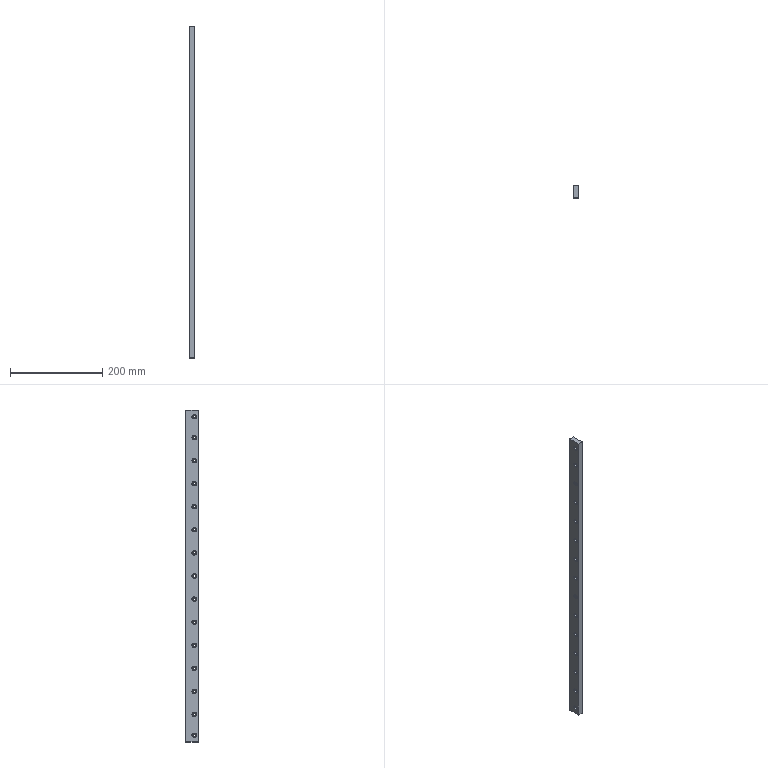Part | SolidWorks | features Chamfer 1, Extrusion 1, HoleWzd 1 | 1 solid | 281 faces | box 12 x 28 x 720 mm | volume 234641 mm3 | plane 161 | cylinder 60 | cone 60 | commonest cylinder face diameters 4.5 x30 8 x30